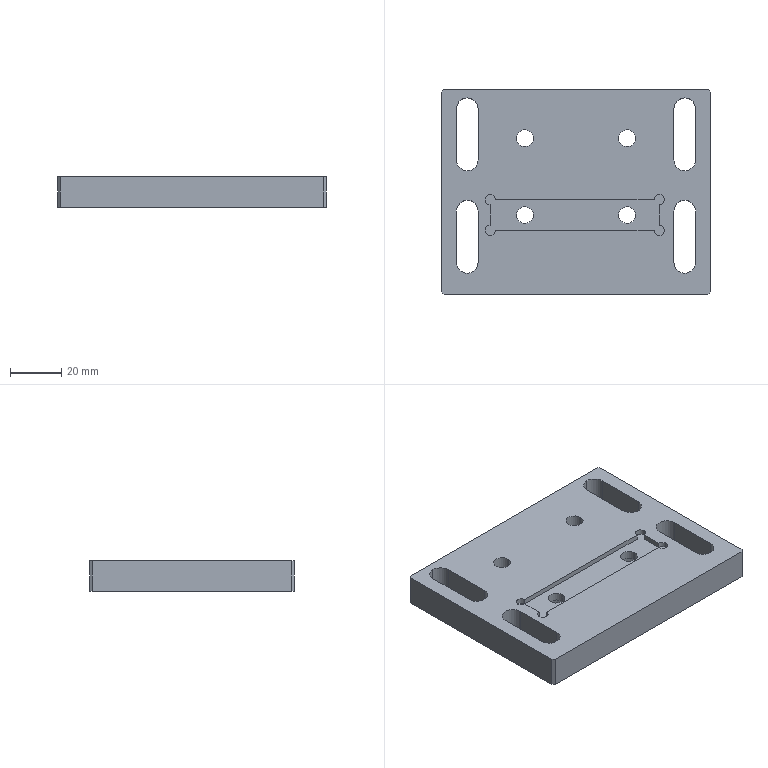CAM job | NX | 3-axis milling, drilling | part box 105 x 80 x 12 mm | stock box 105 x 80 x 12 mm
Tools:
number,name,description,diameter,corner_radius,flute_length,length,flutes
7,D6A45,Milling Tool-5 Parameters,6.0,0.0,3.0,3.0,2
16,6.6ZT,Drilling Tool,6.8,0.0,35.0,50.0,2
14,4.0ZT,Drilling Tool,4.0,0.0,35.0,50.0,2
6,D6,Milling Tool-5 Parameters,6.0,0.0,50.0,75.0,2
4,D4,Milling Tool-5 Parameters,4.0,0.0,50.0,75.0,2
Operations:
program,operation,operation_type,tool,method,geometry_group,spindle_rpm,surface_speed,feed_per_tooth,feed_cut,feed_plunge,cut_length_mm,path_length_mm,cut_time_min,machine_time_min
1-80-105-12毛胚,DRILLING_COPY_1,Operation,D6A45,METHOD,A,3000.0,56.0,0.0333,200.0,0.0,32.0,294.037,0.16,0.1862
1-80-105-12毛胚,DRILLING_COPY_1_COPY,Operation,6.6ZT,METHOD,A,2000.0,42.0,0.05,200.0,0.0,74.172,317.755,0.3709,0.3952
1-80-105-12毛胚,DRILLING_COPY_1_COPY_COPY,Operation,4.0ZT,METHOD,A,2000.0,42.0,0.05,200.0,0.0,24.807,263.119,0.124,0.1479
1-80-105-12毛胚,ZLEVEL_PROFILE_COPY_1_COPY,ZLevelMilling,D6,METHOD,A,7500.0,141.0,0.12,1800.0,100.0,4102.242,4551.086,2.279,2.324
1-80-105-12毛胚,ZLEVEL_PROFILE_COPY_1_COPY_COPY,ZLevelMilling,D6,METHOD,A,7500.0,141.0,0.12,1800.0,100.0,593.169,652.169,0.3295,0.3354
1-80-105-12毛胚,ZLEVEL_PROFILE_COPY_COPY_1,ZLevelMilling,D6,METHOD,A,8000.0,251.0,0.05,800.0,100.0,213.418,725.882,0.2668,0.318
1-80-105-12毛胚,ZLEVEL_PROFILE_COPY_1_COPY_1_COPY_1_1_COPY_COPY,ZLevelMilling,D4,METHOD,A,8000.0,100.0,0.0875,1400.0,800.0,96.428,439.794,0.0808,0.1151
1-80-105-12毛胚,FLOOR_WALL_1_COPY_1,VolumeBased25DMillingOperation,D4,METHOD,A,7500.0,94.0,0.0733,1100.0,100.0,379.838,440.838,0.3453,0.3514
1-80-105-12毛胚,ZLEVEL_PROFILE_1_COPY_1_COPY_COPY_1_COPY,ZLevelMilling,D6A45,METHOD,A,7500.0,141.0,0.0667,1000.0,100.0,481.37,1369.877,0.4814,0.5702